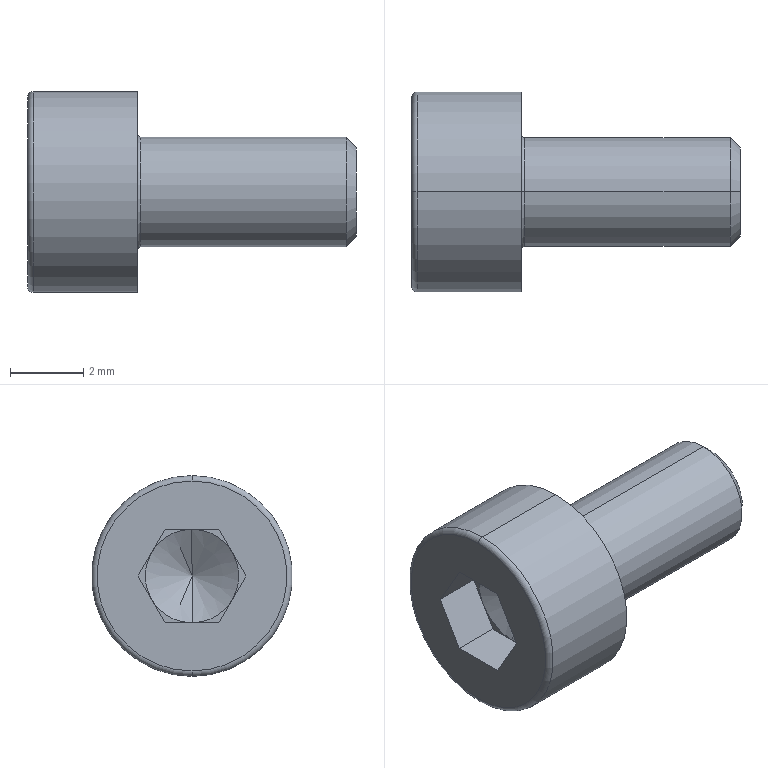Part | SolidWorks | features Fillet 2, RevCut 2, Cut 1, LPattern 1, Revolution 1 | 1 solid | 27 faces | box 9 x 5.5 x 5.5 mm | volume 104.631 mm3 | plane 15 | cone 4 | torus 4 | cylinder 4 | commonest cylinder face diameters 3 x2 5.5 x2
STEP:
#1=CARTESIAN_POINT('',(2.039,0.,0.));
#2=VERTEX_POINT('',#1);
#3=CARTESIAN_POINT('',(1.3,0.,1.28));
#4=VERTEX_POINT('',#3);
#5=CARTESIAN_POINT('',(1.3,0.,1.28));
#6=DIRECTION('',(-0.5,0.,0.866));
#7=VECTOR('',#6,1000.);
#8=LINE('',#5,#7);
#9=EDGE_CURVE('',#2,#4,#8,.T.);
#10=ORIENTED_EDGE('',*,*,#9,.F.);
#11=CARTESIAN_POINT('',(1.3,0.,-1.28));
#12=VERTEX_POINT('',#11);
#13=CARTESIAN_POINT('',(1.3,0.,-1.28));
#14=DIRECTION('',(-0.5,0.,-0.866));
#15=VECTOR('',#14,1000.);
#16=LINE('',#13,#15);
#17=EDGE_CURVE('',#2,#12,#16,.T.);
#18=ORIENTED_EDGE('',*,*,#17,.T.);
#19=CARTESIAN_POINT('',(1.3,-1.109,-0.64));
#20=VERTEX_POINT('',#19);
#21=CARTESIAN_POINT('',(1.3,0.,0.));
#22=DIRECTION('',(-1.,0.,0.));
#23=DIRECTION('',(0.,0.,1.));
#24=AXIS2_PLACEMENT_3D('',#21,#22,#23);
#25=CIRCLE('',#24,1.28);
#26=EDGE_CURVE('',#12,#20,#25,.T.);
#27=ORIENTED_EDGE('',*,*,#26,.T.);
#28=CARTESIAN_POINT('',(1.3,-1.109,0.64));
#29=VERTEX_POINT('',#28);
#30=CARTESIAN_POINT('',(1.3,0.,0.));
#31=DIRECTION('',(-1.,0.,0.));
#32=DIRECTION('',(0.,0.,1.));
#33=AXIS2_PLACEMENT_3D('',#30,#31,#32);
#34=CIRCLE('',#33,1.28);
#35=EDGE_CURVE('',#20,#29,#34,.T.);
#36=ORIENTED_EDGE('',*,*,#35,.T.);
#37=CARTESIAN_POINT('',(1.3,0.,0.));
#38=DIRECTION('',(-1.,0.,0.));
#39=DIRECTION('',(0.,0.,1.));
#40=AXIS2_PLACEMENT_3D('',#37,#38,#39);
#41=CIRCLE('',#40,1.28);
#42=EDGE_CURVE('',#29,#4,#41,.T.);
#43=ORIENTED_EDGE('',*,*,#42,.T.);
#44=EDGE_LOOP('',(#10,#18,#27,#36,#43));
#45=FACE_OUTER_BOUND('',#44,.T.);
#46=CARTESIAN_POINT('',(1.3,0.,0.));
#47=DIRECTION('',(-1.,0.,0.));
#48=DIRECTION('',(0.,0.,1.));
#49=AXIS2_PLACEMENT_3D('',#46,#47,#48);
#50=CONICAL_SURFACE('',#49,1.28,1.047);
#51=ADVANCED_FACE('',(#45),#50,.F.);
#52=CARTESIAN_POINT('',(0.15,0.,-2.75));
#53=VERTEX_POINT('',#52);
#54=CARTESIAN_POINT('',(0.15,0.,2.75));
#55=VERTEX_POINT('',#54);
#56=CARTESIAN_POINT('',(0.15,0.,0.));
#57=DIRECTION('',(1.,0.,0.));
#58=DIRECTION('',(0.,0.,1.));
#59=AXIS2_PLACEMENT_3D('',#56,#57,#58);
#60=CIRCLE('',#59,2.75);
#61=EDGE_CURVE('',#53,#55,#60,.T.);
#62=ORIENTED_EDGE('',*,*,#61,.F.);
#63=CARTESIAN_POINT('',(0.,0.,-2.6));
#64=VERTEX_POINT('',#63);
#65=CARTESIAN_POINT('',(0.15,0.,-2.6));
#66=DIRECTION('',(0.,1.,0.));
#67=DIRECTION('',(0.,0.,1.));
#68=AXIS2_PLACEMENT_3D('',#65,#66,#67);
#69=CIRCLE('',#68,0.15);
#70=EDGE_CURVE('',#53,#64,#69,.T.);
#71=ORIENTED_EDGE('',*,*,#70,.T.);
#72=CARTESIAN_POINT('',(0.,0.,2.6));
#73=VERTEX_POINT('',#72);
#74=CARTESIAN_POINT('',(0.,0.,0.));
#75=DIRECTION('',(-1.,0.,0.));
#76=DIRECTION('',(0.,0.,1.));
#77=AXIS2_PLACEMENT_3D('',#74,#75,#76);
#78=CIRCLE('',#77,2.6);
#79=EDGE_CURVE('',#73,#64,#78,.T.);
#80=ORIENTED_EDGE('',*,*,#79,.F.);
#81=CARTESIAN_POINT('',(0.15,0.,2.6));
#82=DIRECTION('',(0.,-1.,0.));
#83=DIRECTION('',(0.,0.,-1.));
#84=AXIS2_PLACEMENT_3D('',#81,#82,#83);
#85=CIRCLE('',#84,0.15);
#86=EDGE_CURVE('',#55,#73,#85,.T.);
#87=ORIENTED_EDGE('',*,*,#86,.F.);
#88=EDGE_LOOP('',(#62,#71,#80,#87));
#89=FACE_OUTER_BOUND('',#88,.T.);
#90=CARTESIAN_POINT('',(0.15,0.,0.));
#91=DIRECTION('',(-1.,0.,0.));
#92=DIRECTION('',(0.,0.,1.));
#93=AXIS2_PLACEMENT_3D('',#90,#91,#92);
#94=TOROIDAL_SURFACE('',#93,2.6,0.15);
#95=ADVANCED_FACE('',(#89),#94,.T.);
#96=CARTESIAN_POINT('',(3.1,0.,1.5));
#97=VERTEX_POINT('',#96);
#98=CARTESIAN_POINT('',(3.1,0.,-1.5));
#99=VERTEX_POINT('',#98);
#100=CARTESIAN_POINT('',(3.1,0.,0.));
#101=DIRECTION('',(1.,0.,0.));
#102=DIRECTION('',(0.,0.,-1.));
#103=AXIS2_PLACEMENT_3D('',#100,#101,#102);
#104=CIRCLE('',#103,1.5);
#105=EDGE_CURVE('',#97,#99,#104,.T.);
#106=ORIENTED_EDGE('',*,*,#105,.F.);
#107=CARTESIAN_POINT('',(3.,0.,1.6));
#108=VERTEX_POINT('',#107);
#109=CARTESIAN_POINT('',(3.1,0.,1.6));
#110=DIRECTION('',(0.,1.,0.));
#111=DIRECTION('',(0.,0.,1.));
#112=AXIS2_PLACEMENT_3D('',#109,#110,#111);
#113=CIRCLE('',#112,0.1);
#114=EDGE_CURVE('',#97,#108,#113,.T.);
#115=ORIENTED_EDGE('',*,*,#114,.T.);
#116=CARTESIAN_POINT('',(3.,0.,-1.6));
#117=VERTEX_POINT('',#116);
#118=CARTESIAN_POINT('',(3.,0.,0.));
#119=DIRECTION('',(-1.,0.,0.));
#120=DIRECTION('',(0.,0.,-1.));
#121=AXIS2_PLACEMENT_3D('',#118,#119,#120);
#122=CIRCLE('',#121,1.6);
#123=EDGE_CURVE('',#117,#108,#122,.T.);
#124=ORIENTED_EDGE('',*,*,#123,.F.);
#125=CARTESIAN_POINT('',(3.1,0.,-1.6));
#126=DIRECTION('',(0.,-1.,0.));
#127=DIRECTION('',(0.,0.,-1.));
#128=AXIS2_PLACEMENT_3D('',#125,#126,#127);
#129=CIRCLE('',#128,0.1);
#130=EDGE_CURVE('',#99,#117,#129,.T.);
#131=ORIENTED_EDGE('',*,*,#130,.F.);
#132=EDGE_LOOP('',(#106,#115,#124,#131));
#133=FACE_OUTER_BOUND('',#132,.T.);
#134=CARTESIAN_POINT('',(3.1,0.,0.));
#135=DIRECTION('',(1.,0.,0.));
#136=DIRECTION('',(0.,0.,-1.));
#137=AXIS2_PLACEMENT_3D('',#134,#135,#136);
#138=TOROIDAL_SURFACE('',#137,1.6,0.1);
#139=ADVANCED_FACE('',(#133),#138,.F.);
#140=CARTESIAN_POINT('',(9.,0.,1.22));
#141=VERTEX_POINT('',#140);
#142=CARTESIAN_POINT('',(9.,0.,-1.22));
#143=VERTEX_POINT('',#142);
#144=CARTESIAN_POINT('',(9.,0.,0.));
#145=DIRECTION('',(-1.,0.,0.));
#146=DIRECTION('',(0.,0.,1.));
#147=AXIS2_PLACEMENT_3D('',#144,#145,#146);
#148=CIRCLE('',#147,1.22);
#149=EDGE_CURVE('',#141,#143,#148,.T.);
#150=ORIENTED_EDGE('',*,*,#149,.T.);
#151=CARTESIAN_POINT('',(8.72,0.,-1.5));
#152=VERTEX_POINT('',#151);
#153=CARTESIAN_POINT('',(9.,0.,-1.22));
#154=DIRECTION('',(-0.7071,0.,-0.7071));
#155=VECTOR('',#154,1000.);
#156=LINE('',#153,#155);
#157=EDGE_CURVE('',#143,#152,#156,.T.);
#158=ORIENTED_EDGE('',*,*,#157,.T.);
#159=CARTESIAN_POINT('',(8.72,0.,1.5));
#160=VERTEX_POINT('',#159);
#161=CARTESIAN_POINT('',(8.72,0.,0.));
#162=DIRECTION('',(-1.,0.,0.));
#163=DIRECTION('',(0.,0.,1.));
#164=AXIS2_PLACEMENT_3D('',#161,#162,#163);
#165=CIRCLE('',#164,1.5);
#166=EDGE_CURVE('',#160,#152,#165,.T.);
#167=ORIENTED_EDGE('',*,*,#166,.F.);
#168=CARTESIAN_POINT('',(9.,0.,1.22));
#169=DIRECTION('',(-0.7071,0.,0.7071));
#170=VECTOR('',#169,1000.);
#171=LINE('',#168,#170);
#172=EDGE_CURVE('',#141,#160,#171,.T.);
#173=ORIENTED_EDGE('',*,*,#172,.F.);
#174=EDGE_LOOP('',(#150,#158,#167,#173));
#175=FACE_OUTER_BOUND('',#174,.T.);
#176=CARTESIAN_POINT('',(9.,0.,0.));
#177=DIRECTION('',(-1.,0.,0.));
#178=DIRECTION('',(0.,0.,1.));
#179=AXIS2_PLACEMENT_3D('',#176,#177,#178);
#180=CONICAL_SURFACE('',#179,1.22,0.7854);
#181=ADVANCED_FACE('',(#175),#180,.T.);
#182=ORIENTED_EDGE('',*,*,#166,.T.);
#183=CARTESIAN_POINT('',(-31.75,0.,-1.5));
#184=DIRECTION('',(-1.,0.,0.));
#185=VECTOR('',#184,1000.);
#186=LINE('',#183,#185);
#187=EDGE_CURVE('',#152,#99,#186,.T.);
#188=ORIENTED_EDGE('',*,*,#187,.T.);
#189=CARTESIAN_POINT('',(3.1,0.,0.));
#190=DIRECTION('',(1.,0.,0.));
#191=DIRECTION('',(0.,0.,-1.));
#192=AXIS2_PLACEMENT_3D('',#189,#190,#191);
#193=CIRCLE('',#192,1.5);
#194=EDGE_CURVE('',#99,#97,#193,.T.);
#195=ORIENTED_EDGE('',*,*,#194,.T.);
#196=CARTESIAN_POINT('',(-31.75,0.,1.5));
#197=DIRECTION('',(-1.,0.,0.));
#198=VECTOR('',#197,1000.);
#199=LINE('',#196,#198);
#200=EDGE_CURVE('',#160,#97,#199,.T.);
#201=ORIENTED_EDGE('',*,*,#200,.F.);
#202=EDGE_LOOP('',(#182,#188,#195,#201));
#203=FACE_OUTER_BOUND('',#202,.T.);
#204=CARTESIAN_POINT('',(-31.75,0.,0.));
#205=DIRECTION('',(-1.,0.,0.));
#206=DIRECTION('',(0.,0.,1.));
#207=AXIS2_PLACEMENT_3D('',#204,#205,#206);
#208=CYLINDRICAL_SURFACE('',#207,1.5);
#209=ADVANCED_FACE('',(#203),#208,.T.);
#210=CARTESIAN_POINT('',(3.,0.,2.75));
#211=VERTEX_POINT('',#210);
#212=CARTESIAN_POINT('',(3.,0.,-2.75));
#213=VERTEX_POINT('',#212);
#214=CARTESIAN_POINT('',(3.,0.,0.));
#215=DIRECTION('',(-1.,0.,0.));
#216=DIRECTION('',(0.,0.,1.));
#217=AXIS2_PLACEMENT_3D('',#214,#215,#216);
#218=CIRCLE('',#217,2.75);
#219=EDGE_CURVE('',#211,#213,#218,.T.);
#220=ORIENTED_EDGE('',*,*,#219,.T.);
#221=CARTESIAN_POINT('',(-31.75,0.,-2.75));
#222=DIRECTION('',(-1.,0.,0.));
#223=VECTOR('',#222,1000.);
#224=LINE('',#221,#223);
#225=EDGE_CURVE('',#213,#53,#224,.T.);
#226=ORIENTED_EDGE('',*,*,#225,.T.);
#227=ORIENTED_EDGE('',*,*,#61,.T.);
#228=CARTESIAN_POINT('',(-31.75,0.,2.75));
#229=DIRECTION('',(-1.,0.,0.));
#230=VECTOR('',#229,1000.);
#231=LINE('',#228,#230);
#232=EDGE_CURVE('',#211,#55,#231,.T.);
#233=ORIENTED_EDGE('',*,*,#232,.F.);
#234=EDGE_LOOP('',(#220,#226,#227,#233));
#235=FACE_OUTER_BOUND('',#234,.T.);
#236=CARTESIAN_POINT('',(-31.75,0.,0.));
#237=DIRECTION('',(-1.,0.,0.));
#238=DIRECTION('',(0.,0.,1.));
#239=AXIS2_PLACEMENT_3D('',#236,#237,#238);
#240=CYLINDRICAL_SURFACE('',#239,2.75);
#241=ADVANCED_FACE('',(#235),#240,.T.);
#242=CARTESIAN_POINT('',(0.,1.478,0.));
#243=VERTEX_POINT('',#242);
#244=CARTESIAN_POINT('',(0.,0.739,1.28));
#245=VERTEX_POINT('',#244);
#246=CARTESIAN_POINT('',(0.,1.478,0.));
#247=DIRECTION('',(0.,-0.5,0.866));
#248=VECTOR('',#247,1000.);
#249=LINE('',#246,#248);
#250=EDGE_CURVE('',#243,#245,#249,.T.);
#251=ORIENTED_EDGE('',*,*,#250,.T.);
#252=CARTESIAN_POINT('',(0.,-0.739,1.28));
#253=VERTEX_POINT('',#252);
#254=CARTESIAN_POINT('',(0.,-0.739,1.28));
#255=DIRECTION('',(0.,1.,0.));
#256=VECTOR('',#255,1000.);
#257=LINE('',#254,#256);
#258=EDGE_CURVE('',#253,#245,#257,.T.);
#259=ORIENTED_EDGE('',*,*,#258,.F.);
#260=CARTESIAN_POINT('',(0.,-1.478,0.));
#261=VERTEX_POINT('',#260);
#262=CARTESIAN_POINT('',(0.,-0.739,1.28));
#263=DIRECTION('',(0.,-0.5,-0.866));
#264=VECTOR('',#263,1000.);
#265=LINE('',#262,#264);
#266=EDGE_CURVE('',#253,#261,#265,.T.);
#267=ORIENTED_EDGE('',*,*,#266,.T.);
#268=CARTESIAN_POINT('',(0.,-0.739,-1.28));
#269=VERTEX_POINT('',#268);
#270=CARTESIAN_POINT('',(0.,-1.478,0.));
#271=DIRECTION('',(0.,0.5,-0.866));
#272=VECTOR('',#271,1000.);
#273=LINE('',#270,#272);
#274=EDGE_CURVE('',#261,#269,#273,.T.);
#275=ORIENTED_EDGE('',*,*,#274,.T.);
#276=CARTESIAN_POINT('',(0.,0.739,-1.28));
#277=VERTEX_POINT('',#276);
#278=CARTESIAN_POINT('',(0.,0.739,-1.28));
#279=DIRECTION('',(0.,-1.,0.));
#280=VECTOR('',#279,1000.);
#281=LINE('',#278,#280);
#282=EDGE_CURVE('',#277,#269,#281,.T.);
#283=ORIENTED_EDGE('',*,*,#282,.F.);
#284=CARTESIAN_POINT('',(0.,1.478,0.));
#285=DIRECTION('',(0.,-0.5,-0.866));
#286=VECTOR('',#285,1000.);
#287=LINE('',#284,#286);
#288=EDGE_CURVE('',#243,#277,#287,.T.);
#289=ORIENTED_EDGE('',*,*,#288,.F.);
#290=EDGE_LOOP('',(#251,#259,#267,#275,#283,#289));
#291=FACE_BOUND('',#290,.T.);
#292=ORIENTED_EDGE('',*,*,#79,.T.);
#293=CARTESIAN_POINT('',(0.,0.,0.));
#294=DIRECTION('',(-1.,0.,0.));
#295=DIRECTION('',(0.,0.,1.));
#296=AXIS2_PLACEMENT_3D('',#293,#294,#295);
#297=CIRCLE('',#296,2.6);
#298=EDGE_CURVE('',#64,#73,#297,.T.);
#299=ORIENTED_EDGE('',*,*,#298,.T.);
#300=EDGE_LOOP('',(#292,#299));
#301=FACE_OUTER_BOUND('',#300,.T.);
#302=CARTESIAN_POINT('',(0.,0.,0.));
#303=DIRECTION('',(-1.,0.,0.));
#304=DIRECTION('',(0.,0.,1.));
#305=AXIS2_PLACEMENT_3D('',#302,#303,#304);
#306=PLANE('',#305);
#307=ADVANCED_FACE('',(#291,#301),#306,.T.);
#308=ORIENTED_EDGE('',*,*,#225,.F.);
#309=CARTESIAN_POINT('',(3.,0.,0.));
#310=DIRECTION('',(-1.,0.,0.));
#311=DIRECTION('',(0.,0.,1.));
#312=AXIS2_PLACEMENT_3D('',#309,#310,#311);
#313=CIRCLE('',#312,2.75);
#314=EDGE_CURVE('',#213,#211,#313,.T.);
#315=ORIENTED_EDGE('',*,*,#314,.T.);
#316=ORIENTED_EDGE('',*,*,#232,.T.);
#317=CARTESIAN_POINT('',(0.15,0.,0.));
#318=DIRECTION('',(1.,0.,0.));
#319=DIRECTION('',(0.,0.,1.));
#320=AXIS2_PLACEMENT_3D('',#317,#318,#319);
#321=CIRCLE('',#320,2.75);
#322=EDGE_CURVE('',#55,#53,#321,.T.);
#323=ORIENTED_EDGE('',*,*,#322,.T.);
#324=EDGE_LOOP('',(#308,#315,#316,#323));
#325=FACE_OUTER_BOUND('',#324,.T.);
#326=CARTESIAN_POINT('',(-31.75,0.,0.));
#327=DIRECTION('',(-1.,0.,0.));
#328=DIRECTION('',(0.,0.,1.));
#329=AXIS2_PLACEMENT_3D('',#326,#327,#328);
#330=CYLINDRICAL_SURFACE('',#329,2.75);
#331=ADVANCED_FACE('',(#325),#330,.T.);
#332=ORIENTED_EDGE('',*,*,#123,.T.);
#333=CARTESIAN_POINT('',(3.,0.,0.));
#334=DIRECTION('',(-1.,0.,0.));
#335=DIRECTION('',(0.,0.,-1.));
#336=AXIS2_PLACEMENT_3D('',#333,#334,#335);
#337=CIRCLE('',#336,1.6);
#338=EDGE_CURVE('',#108,#117,#337,.T.);
#339=ORIENTED_EDGE('',*,*,#338,.T.);
#340=EDGE_LOOP('',(#332,#339));
#341=FACE_BOUND('',#340,.T.);
#342=ORIENTED_EDGE('',*,*,#219,.F.);
#343=ORIENTED_EDGE('',*,*,#314,.F.);
#344=EDGE_LOOP('',(#342,#343));
#345=FACE_OUTER_BOUND('',#344,.T.);
#346=CARTESIAN_POINT('',(3.,2.75,0.));
#347=DIRECTION('',(1.,0.,0.));
#348=DIRECTION('',(0.,0.,-1.));
#349=AXIS2_PLACEMENT_3D('',#346,#347,#348);
#350=PLANE('',#349);
#351=ADVANCED_FACE('',(#341,#345),#350,.T.);
#352=ORIENTED_EDGE('',*,*,#187,.F.);
#353=CARTESIAN_POINT('',(8.72,0.,0.));
#354=DIRECTION('',(-1.,0.,0.));
#355=DIRECTION('',(0.,0.,1.));
#356=AXIS2_PLACEMENT_3D('',#353,#354,#355);
#357=CIRCLE('',#356,1.5);
#358=EDGE_CURVE('',#152,#160,#357,.T.);
#359=ORIENTED_EDGE('',*,*,#358,.T.);
#360=ORIENTED_EDGE('',*,*,#200,.T.);
#361=ORIENTED_EDGE('',*,*,#105,.T.);
#362=EDGE_LOOP('',(#352,#359,#360,#361));
#363=FACE_OUTER_BOUND('',#362,.T.);
#364=CARTESIAN_POINT('',(-31.75,0.,0.));
#365=DIRECTION('',(-1.,0.,0.));
#366=DIRECTION('',(0.,0.,1.));
#367=AXIS2_PLACEMENT_3D('',#364,#365,#366);
#368=CYLINDRICAL_SURFACE('',#367,1.5);
#369=ADVANCED_FACE('',(#363),#368,.T.);
#370=ORIENTED_EDGE('',*,*,#157,.F.);
#371=CARTESIAN_POINT('',(9.,0.,0.));
#372=DIRECTION('',(-1.,0.,0.));
#373=DIRECTION('',(0.,0.,1.));
#374=AXIS2_PLACEMENT_3D('',#371,#372,#373);
#375=CIRCLE('',#374,1.22);
#376=EDGE_CURVE('',#143,#141,#375,.T.);
#377=ORIENTED_EDGE('',*,*,#376,.T.);
#378=ORIENTED_EDGE('',*,*,#172,.T.);
#379=ORIENTED_EDGE('',*,*,#358,.F.);
#380=EDGE_LOOP('',(#370,#377,#378,#379));
#381=FACE_OUTER_BOUND('',#380,.T.);
#382=CARTESIAN_POINT('',(9.,0.,0.));
#383=DIRECTION('',(-1.,0.,0.));
#384=DIRECTION('',(0.,0.,1.));
#385=AXIS2_PLACEMENT_3D('',#382,#383,#384);
#386=CONICAL_SURFACE('',#385,1.22,0.7854);
#387=ADVANCED_FACE('',(#381),#386,.T.);
#388=ORIENTED_EDGE('',*,*,#149,.F.);
#389=ORIENTED_EDGE('',*,*,#376,.F.);
#390=EDGE_LOOP('',(#388,#389));
#391=FACE_OUTER_BOUND('',#390,.T.);
#392=CARTESIAN_POINT('',(9.,1.22,0.));
#393=DIRECTION('',(1.,0.,0.));
#394=DIRECTION('',(0.,0.,-1.));
#395=AXIS2_PLACEMENT_3D('',#392,#393,#394);
#396=PLANE('',#395);
#397=ADVANCED_FACE('',(#391),#396,.T.);
#398=ORIENTED_EDGE('',*,*,#114,.F.);
#399=ORIENTED_EDGE('',*,*,#194,.F.);
#400=ORIENTED_EDGE('',*,*,#130,.T.);
#401=ORIENTED_EDGE('',*,*,#338,.F.);
#402=EDGE_LOOP('',(#398,#399,#400,#401));
#403=FACE_OUTER_BOUND('',#402,.T.);
#404=CARTESIAN_POINT('',(3.1,0.,0.));
#405=DIRECTION('',(1.,0.,0.));
#406=DIRECTION('',(0.,0.,-1.));
#407=AXIS2_PLACEMENT_3D('',#404,#405,#406);
#408=TOROIDAL_SURFACE('',#407,1.6,0.1);
#409=ADVANCED_FACE('',(#403),#408,.F.);
#410=ORIENTED_EDGE('',*,*,#70,.F.);
#411=ORIENTED_EDGE('',*,*,#322,.F.);
#412=ORIENTED_EDGE('',*,*,#86,.T.);
#413=ORIENTED_EDGE('',*,*,#298,.F.);
#414=EDGE_LOOP('',(#410,#411,#412,#413));
#415=FACE_OUTER_BOUND('',#414,.T.);
#416=CARTESIAN_POINT('',(0.15,0.,0.));
#417=DIRECTION('',(-1.,0.,0.));
#418=DIRECTION('',(0.,0.,1.));
#419=AXIS2_PLACEMENT_3D('',#416,#417,#418);
#420=TOROIDAL_SURFACE('',#419,2.6,0.15);
#421=ADVANCED_FACE('',(#415),#420,.T.);
#422=ORIENTED_EDGE('',*,*,#250,.F.);
#423=CARTESIAN_POINT('',(1.3,1.478,0.));
#424=VERTEX_POINT('',#423);
#425=CARTESIAN_POINT('',(1.3,1.478,0.));
#426=DIRECTION('',(-1.,0.,0.));
#427=VECTOR('',#426,1000.);
#428=LINE('',#425,#427);
#429=EDGE_CURVE('',#424,#243,#428,.T.);
#430=ORIENTED_EDGE('',*,*,#429,.F.);
#431=CARTESIAN_POINT('',(1.3,1.109,0.64));
#432=VERTEX_POINT('',#431);
#433=CARTESIAN_POINT('',(1.3,1.478,0.));
#434=DIRECTION('',(0.,-0.5,0.866));
#435=VECTOR('',#434,1000.);
#436=LINE('',#433,#435);
#437=EDGE_CURVE('',#424,#432,#436,.T.);
#438=ORIENTED_EDGE('',*,*,#437,.T.);
#439=CARTESIAN_POINT('',(1.3,0.739,1.28));
#440=VERTEX_POINT('',#439);
#441=CARTESIAN_POINT('',(1.3,1.478,0.));
#442=DIRECTION('',(0.,-0.5,0.866));
#443=VECTOR('',#442,1000.);
#444=LINE('',#441,#443);
#445=EDGE_CURVE('',#432,#440,#444,.T.);
#446=ORIENTED_EDGE('',*,*,#445,.T.);
#447=CARTESIAN_POINT('',(1.3,0.739,1.28));
#448=DIRECTION('',(-1.,0.,0.));
#449=VECTOR('',#448,1000.);
#450=LINE('',#447,#449);
#451=EDGE_CURVE('',#440,#245,#450,.T.);
#452=ORIENTED_EDGE('',*,*,#451,.T.);
#453=EDGE_LOOP('',(#422,#430,#438,#446,#452));
#454=FACE_OUTER_BOUND('',#453,.T.);
#455=CARTESIAN_POINT('',(1.3,1.478,0.));
#456=DIRECTION('',(0.,-0.866,-0.5));
#457=DIRECTION('',(0.,0.5,-0.866));
#458=AXIS2_PLACEMENT_3D('',#455,#456,#457);
#459=PLANE('',#458);
#460=ADVANCED_FACE('',(#454),#459,.T.);
#461=ORIENTED_EDGE('',*,*,#258,.T.);
#462=ORIENTED_EDGE('',*,*,#451,.F.);
#463=CARTESIAN_POINT('',(1.3,-0.739,1.28));
#464=DIRECTION('',(0.,1.,0.));
#465=VECTOR('',#464,1000.);
#466=LINE('',#463,#465);
#467=EDGE_CURVE('',#4,#440,#466,.T.);
#468=ORIENTED_EDGE('',*,*,#467,.F.);
#469=CARTESIAN_POINT('',(1.3,-0.739,1.28));
#470=VERTEX_POINT('',#469);
#471=CARTESIAN_POINT('',(1.3,-0.739,1.28));
#472=DIRECTION('',(0.,1.,0.));
#473=VECTOR('',#472,1000.);
#474=LINE('',#471,#473);
#475=EDGE_CURVE('',#470,#4,#474,.T.);
#476=ORIENTED_EDGE('',*,*,#475,.F.);
#477=CARTESIAN_POINT('',(1.3,-0.739,1.28));
#478=DIRECTION('',(-1.,0.,0.));
#479=VECTOR('',#478,1000.);
#480=LINE('',#477,#479);
#481=EDGE_CURVE('',#470,#253,#480,.T.);
#482=ORIENTED_EDGE('',*,*,#481,.T.);
#483=EDGE_LOOP('',(#461,#462,#468,#476,#482));
#484=FACE_OUTER_BOUND('',#483,.T.);
#485=CARTESIAN_POINT('',(1.3,-0.739,1.28));
#486=DIRECTION('',(0.,0.,1.));
#487=DIRECTION('',(0.,-1.,0.));
#488=AXIS2_PLACEMENT_3D('',#485,#486,#487);
#489=PLANE('',#488);
#490=ADVANCED_FACE('',(#484),#489,.F.);
#491=ORIENTED_EDGE('',*,*,#266,.F.);
#492=ORIENTED_EDGE('',*,*,#481,.F.);
#493=CARTESIAN_POINT('',(1.3,-0.739,1.28));
#494=DIRECTION('',(0.,-0.5,-0.866));
#495=VECTOR('',#494,1000.);
#496=LINE('',#493,#495);
#497=EDGE_CURVE('',#470,#29,#496,.T.);
#498=ORIENTED_EDGE('',*,*,#497,.T.);
#499=CARTESIAN_POINT('',(1.3,-1.478,0.));
#500=VERTEX_POINT('',#499);
#501=CARTESIAN_POINT('',(1.3,-0.739,1.28));
#502=DIRECTION('',(0.,-0.5,-0.866));
#503=VECTOR('',#502,1000.);
#504=LINE('',#501,#503);
#505=EDGE_CURVE('',#29,#500,#504,.T.);
#506=ORIENTED_EDGE('',*,*,#505,.T.);
#507=CARTESIAN_POINT('',(1.3,-1.478,0.));
#508=DIRECTION('',(-1.,0.,0.));
#509=VECTOR('',#508,1000.);
#510=LINE('',#507,#509);
#511=EDGE_CURVE('',#500,#261,#510,.T.);
#512=ORIENTED_EDGE('',*,*,#511,.T.);
#513=EDGE_LOOP('',(#491,#492,#498,#506,#512));
#514=FACE_OUTER_BOUND('',#513,.T.);
#515=CARTESIAN_POINT('',(1.3,-0.739,1.28));
#516=DIRECTION('',(0.,0.866,-0.5));
#517=DIRECTION('',(0.,0.5,0.866));
#518=AXIS2_PLACEMENT_3D('',#515,#516,#517);
#519=PLANE('',#518);
#520=ADVANCED_FACE('',(#514),#519,.T.);
#521=ORIENTED_EDGE('',*,*,#274,.F.);
#522=ORIENTED_EDGE('',*,*,#511,.F.);
#523=CARTESIAN_POINT('',(1.3,-1.478,0.));
#524=DIRECTION('',(0.,0.5,-0.866));
#525=VECTOR('',#524,1000.);
#526=LINE('',#523,#525);
#527=EDGE_CURVE('',#500,#20,#526,.T.);
#528=ORIENTED_EDGE('',*,*,#527,.T.);
#529=CARTESIAN_POINT('',(1.3,-0.739,-1.28));
#530=VERTEX_POINT('',#529);
#531=CARTESIAN_POINT('',(1.3,-1.478,0.));
#532=DIRECTION('',(0.,0.5,-0.866));
#533=VECTOR('',#532,1000.);
#534=LINE('',#531,#533);
#535=EDGE_CURVE('',#20,#530,#534,.T.);
#536=ORIENTED_EDGE('',*,*,#535,.T.);
#537=CARTESIAN_POINT('',(1.3,-0.739,-1.28));
#538=DIRECTION('',(-1.,0.,0.));
#539=VECTOR('',#538,1000.);
#540=LINE('',#537,#539);
#541=EDGE_CURVE('',#530,#269,#540,.T.);
#542=ORIENTED_EDGE('',*,*,#541,.T.);
#543=EDGE_LOOP('',(#521,#522,#528,#536,#542));
#544=FACE_OUTER_BOUND('',#543,.T.);
#545=CARTESIAN_POINT('',(1.3,-1.478,0.));
#546=DIRECTION('',(0.,0.866,0.5));
#547=DIRECTION('',(0.,-0.5,0.866));
#548=AXIS2_PLACEMENT_3D('',#545,#546,#547);
#549=PLANE('',#548);
#550=ADVANCED_FACE('',(#544),#549,.T.);
#551=ORIENTED_EDGE('',*,*,#282,.T.);
#552=ORIENTED_EDGE('',*,*,#541,.F.);
#553=CARTESIAN_POINT('',(1.3,0.739,-1.28));
#554=DIRECTION('',(0.,-1.,0.));
#555=VECTOR('',#554,1000.);
#556=LINE('',#553,#555);
#557=EDGE_CURVE('',#12,#530,#556,.T.);
#558=ORIENTED_EDGE('',*,*,#557,.F.);
#559=CARTESIAN_POINT('',(1.3,0.739,-1.28));
#560=VERTEX_POINT('',#559);
#561=CARTESIAN_POINT('',(1.3,0.739,-1.28));
#562=DIRECTION('',(0.,-1.,0.));
#563=VECTOR('',#562,1000.);
#564=LINE('',#561,#563);
#565=EDGE_CURVE('',#560,#12,#564,.T.);
#566=ORIENTED_EDGE('',*,*,#565,.F.);
#567=CARTESIAN_POINT('',(1.3,0.739,-1.28));
#568=DIRECTION('',(-1.,0.,0.));
#569=VECTOR('',#568,1000.);
#570=LINE('',#567,#569);
#571=EDGE_CURVE('',#560,#277,#570,.T.);
#572=ORIENTED_EDGE('',*,*,#571,.T.);
#573=EDGE_LOOP('',(#551,#552,#558,#566,#572));
#574=FACE_OUTER_BOUND('',#573,.T.);
#575=CARTESIAN_POINT('',(1.3,0.739,-1.28));
#576=DIRECTION('',(0.,0.,-1.));
#577=DIRECTION('',(0.,1.,0.));
#578=AXIS2_PLACEMENT_3D('',#575,#576,#577);
#579=PLANE('',#578);
#580=ADVANCED_FACE('',(#574),#579,.F.);
#581=ORIENTED_EDGE('',*,*,#288,.T.);
#582=ORIENTED_EDGE('',*,*,#571,.F.);
#583=CARTESIAN_POINT('',(1.3,1.109,-0.64));
#584=VERTEX_POINT('',#583);
#585=CARTESIAN_POINT('',(1.3,1.478,0.));
#586=DIRECTION('',(0.,-0.5,-0.866));
#587=VECTOR('',#586,1000.);
#588=LINE('',#585,#587);
#589=EDGE_CURVE('',#584,#560,#588,.T.);
#590=ORIENTED_EDGE('',*,*,#589,.F.);
#591=CARTESIAN_POINT('',(1.3,1.478,0.));
#592=DIRECTION('',(0.,-0.5,-0.866));
#593=VECTOR('',#592,1000.);
#594=LINE('',#591,#593);
#595=EDGE_CURVE('',#424,#584,#594,.T.);
#596=ORIENTED_EDGE('',*,*,#595,.F.);
#597=ORIENTED_EDGE('',*,*,#429,.T.);
#598=EDGE_LOOP('',(#581,#582,#590,#596,#597));
#599=FACE_OUTER_BOUND('',#598,.T.);
#600=CARTESIAN_POINT('',(1.3,1.478,0.));
#601=DIRECTION('',(0.,0.866,-0.5));
#602=DIRECTION('',(0.,0.5,0.866));
#603=AXIS2_PLACEMENT_3D('',#600,#601,#602);
#604=PLANE('',#603);
#605=ADVANCED_FACE('',(#599),#604,.F.);
#606=ORIENTED_EDGE('',*,*,#557,.T.);
#607=ORIENTED_EDGE('',*,*,#535,.F.);
#608=ORIENTED_EDGE('',*,*,#26,.F.);
#609=EDGE_LOOP('',(#606,#607,#608));
#610=FACE_OUTER_BOUND('',#609,.T.);
#611=CARTESIAN_POINT('',(1.3,2.217,-1.28));
#612=DIRECTION('',(1.,0.,0.));
#613=DIRECTION('',(0.,0.,-1.));
#614=AXIS2_PLACEMENT_3D('',#611,#612,#613);
#615=PLANE('',#614);
#616=ADVANCED_FACE('',(#610),#615,.F.);
#617=ORIENTED_EDGE('',*,*,#527,.F.);
#618=ORIENTED_EDGE('',*,*,#505,.F.);
#619=ORIENTED_EDGE('',*,*,#35,.F.);
#620=EDGE_LOOP('',(#617,#618,#619));
#621=FACE_OUTER_BOUND('',#620,.T.);
#622=CARTESIAN_POINT('',(1.3,2.217,-1.28));
#623=DIRECTION('',(1.,0.,0.));
#624=DIRECTION('',(0.,0.,-1.));
#625=AXIS2_PLACEMENT_3D('',#622,#623,#624);
#626=PLANE('',#625);
#627=ADVANCED_FACE('',(#621),#626,.F.);
#628=ORIENTED_EDGE('',*,*,#497,.F.);
#629=ORIENTED_EDGE('',*,*,#475,.T.);
#630=ORIENTED_EDGE('',*,*,#42,.F.);
#631=EDGE_LOOP('',(#628,#629,#630));
#632=FACE_OUTER_BOUND('',#631,.T.);
#633=CARTESIAN_POINT('',(1.3,2.217,-1.28));
#634=DIRECTION('',(1.,0.,0.));
#635=DIRECTION('',(0.,0.,-1.));
#636=AXIS2_PLACEMENT_3D('',#633,#634,#635);
#637=PLANE('',#636);
#638=ADVANCED_FACE('',(#632),#637,.F.);
#639=ORIENTED_EDGE('',*,*,#467,.T.);
#640=ORIENTED_EDGE('',*,*,#445,.F.);
#641=CARTESIAN_POINT('',(1.3,0.,0.));
#642=DIRECTION('',(-1.,0.,0.));
#643=DIRECTION('',(0.,0.,1.));
#644=AXIS2_PLACEMENT_3D('',#641,#642,#643);
#645=CIRCLE('',#644,1.28);
#646=EDGE_CURVE('',#4,#432,#645,.T.);
#647=ORIENTED_EDGE('',*,*,#646,.F.);
#648=EDGE_LOOP('',(#639,#640,#647));
#649=FACE_OUTER_BOUND('',#648,.T.);
#650=CARTESIAN_POINT('',(1.3,2.217,-1.28));
#651=DIRECTION('',(1.,0.,0.));
#652=DIRECTION('',(0.,0.,-1.));
#653=AXIS2_PLACEMENT_3D('',#650,#651,#652);
#654=PLANE('',#653);
#655=ADVANCED_FACE('',(#649),#654,.F.);
#656=ORIENTED_EDGE('',*,*,#437,.F.);
#657=ORIENTED_EDGE('',*,*,#595,.T.);
#658=CARTESIAN_POINT('',(1.3,0.,0.));
#659=DIRECTION('',(-1.,0.,0.));
#660=DIRECTION('',(0.,0.,1.));
#661=AXIS2_PLACEMENT_3D('',#658,#659,#660);
#662=CIRCLE('',#661,1.28);
#663=EDGE_CURVE('',#432,#584,#662,.T.);
#664=ORIENTED_EDGE('',*,*,#663,.F.);
#665=EDGE_LOOP('',(#656,#657,#664));
#666=FACE_OUTER_BOUND('',#665,.T.);
#667=CARTESIAN_POINT('',(1.3,2.217,-1.28));
#668=DIRECTION('',(1.,0.,0.));
#669=DIRECTION('',(0.,0.,-1.));
#670=AXIS2_PLACEMENT_3D('',#667,#668,#669);
#671=PLANE('',#670);
#672=ADVANCED_FACE('',(#666),#671,.F.);
#673=ORIENTED_EDGE('',*,*,#589,.T.);
#674=ORIENTED_EDGE('',*,*,#565,.T.);
#675=CARTESIAN_POINT('',(1.3,0.,0.));
#676=DIRECTION('',(-1.,0.,0.));
#677=DIRECTION('',(0.,0.,1.));
#678=AXIS2_PLACEMENT_3D('',#675,#676,#677);
#679=CIRCLE('',#678,1.28);
#680=EDGE_CURVE('',#584,#12,#679,.T.);
#681=ORIENTED_EDGE('',*,*,#680,.F.);
#682=EDGE_LOOP('',(#673,#674,#681));
#683=FACE_OUTER_BOUND('',#682,.T.);
#684=CARTESIAN_POINT('',(1.3,2.217,-1.28));
#685=DIRECTION('',(1.,0.,0.));
#686=DIRECTION('',(0.,0.,-1.));
#687=AXIS2_PLACEMENT_3D('',#684,#685,#686);
#688=PLANE('',#687);
#689=ADVANCED_FACE('',(#683),#688,.F.);
#690=ORIENTED_EDGE('',*,*,#17,.F.);
#691=ORIENTED_EDGE('',*,*,#9,.T.);
#692=ORIENTED_EDGE('',*,*,#646,.T.);
#693=ORIENTED_EDGE('',*,*,#663,.T.);
#694=ORIENTED_EDGE('',*,*,#680,.T.);
#695=EDGE_LOOP('',(#690,#691,#692,#693,#694));
#696=FACE_OUTER_BOUND('',#695,.T.);
#697=CARTESIAN_POINT('',(1.3,0.,0.));
#698=DIRECTION('',(-1.,0.,0.));
#699=DIRECTION('',(0.,0.,1.));
#700=AXIS2_PLACEMENT_3D('',#697,#698,#699);
#701=CONICAL_SURFACE('',#700,1.28,1.047);
#702=ADVANCED_FACE('',(#696),#701,.F.);
#703=CLOSED_SHELL('',(#51,#95,#139,#181,#209,#241,#307,#331,#351,#369,#387,#397,#409,#421,#460,#490,#520,#550,#580,#605,#616,#627,#638,#655,#672,#689,#702));
#704=MANIFOLD_SOLID_BREP('',#703);
#705=CARTESIAN_POINT('',(0.,0.,0.));
#706=DIRECTION('',(0.,0.,1.));
#707=DIRECTION('',(1.,0.,0.));
#708=AXIS2_PLACEMENT_3D('',#705,#706,#707);
#709=(LENGTH_UNIT()NAMED_UNIT(*)SI_UNIT(.MILLI.,.METRE.));
#710=UNCERTAINTY_MEASURE_WITH_UNIT(LENGTH_MEASURE(0.00001),#709,'','');
#711=(NAMED_UNIT(*)PLANE_ANGLE_UNIT()SI_UNIT($,.RADIAN.));
#712=(NAMED_UNIT(*)SI_UNIT($,.STERADIAN.)SOLID_ANGLE_UNIT());
#713=(GEOMETRIC_REPRESENTATION_CONTEXT(3)GLOBAL_UNCERTAINTY_ASSIGNED_CONTEXT((#710))GLOBAL_UNIT_ASSIGNED_CONTEXT((#709,#711,#712))REPRESENTATION_CONTEXT('',''));
#714=ADVANCED_BREP_SHAPE_REPRESENTATION('',(#704,#708),#713);